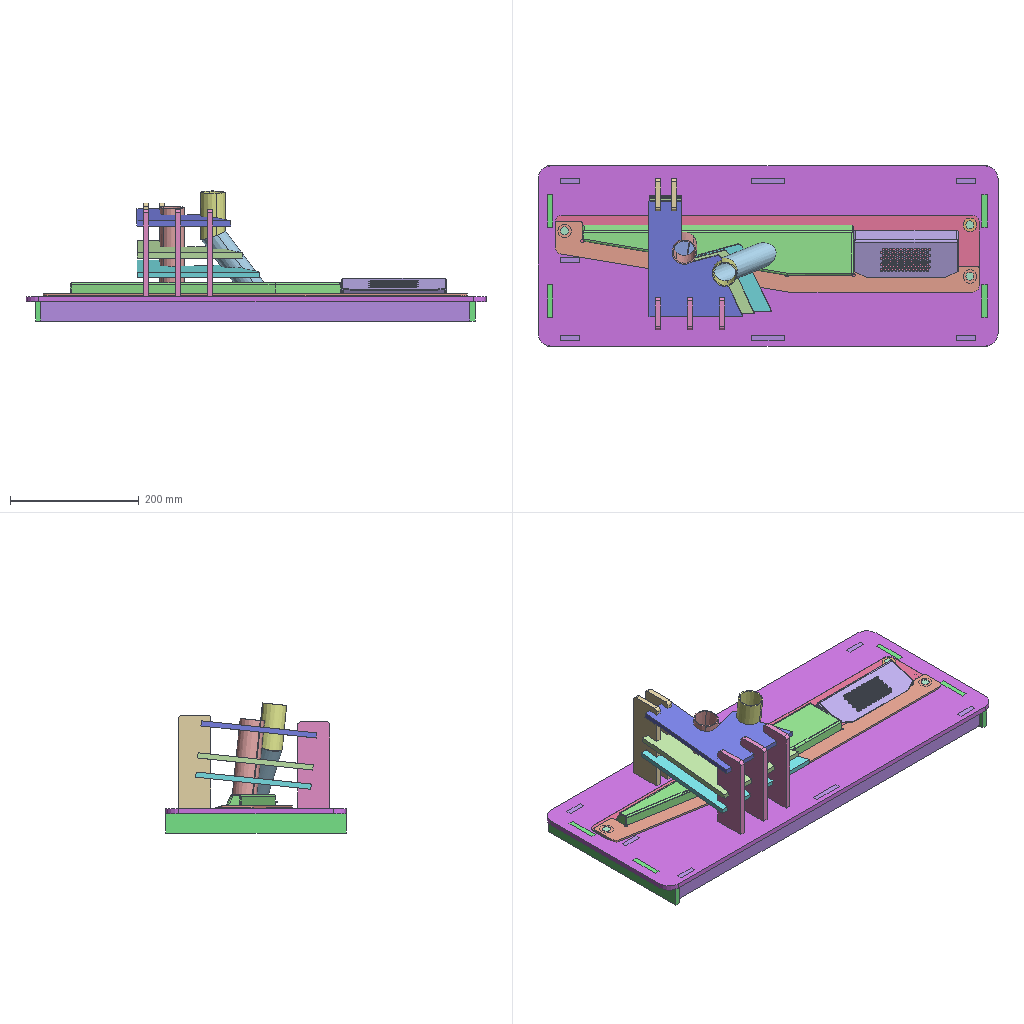Assembly | SolidWorks | 11 different items | 19 placed | box 715 x 280 x 202 mm
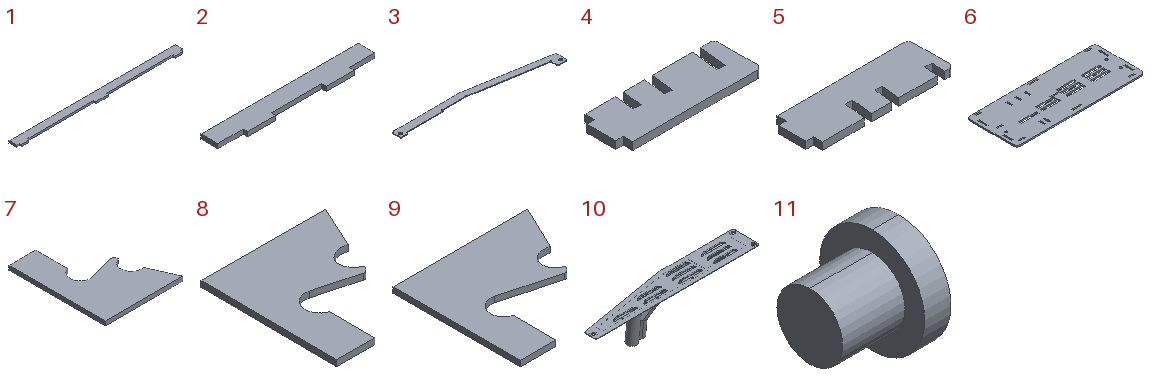Parts list (item | quantity | size | volume | features):
1 | x3 | 667 x 38 x 8 mm | 167120 mm3 | features FlatPattern 1, ICE 1, SMBaseFlange 1, SheetMetal 1
2 | x2 | 280 x 38 x 8 mm | 73600 mm3 | features FlatPattern 1, SMBaseFlange 1, SheetMetal 1
3 | x1 | 659 x 110.2 x 3 mm | 58163 mm3 | features Fillet 2, FlatPattern 1, SMBaseFlange 1, SheetMetal 1
4 | x3 | 143 x 50 x 8 mm | 51129 mm3 | features Fillet 1, FlatPattern 1, SMBaseFlange 1, SheetMetal 1
5 | x2 | 153 x 50 x 8 mm | 56042 mm3 | features Fillet 1, FlatPattern 1, SMBaseFlange 1, SheetMetal 1
6 | x1 | 715 x 280 x 8 mm | 1446309 mm3 | features FlatPattern 1, SMBaseFlange 1, SheetMetal 1
7 | x1 | 145.357 x 180 x 8 mm | 119080 mm3 | features FlatPattern 1, SMBaseFlange 1, SheetMetal 1
8 | x1 | 164.239 x 180.27 x 8 mm | 131142 mm3 | features FlatPattern 1, SMBaseFlange 1, SheetMetal 1
9 | x1 | 190.337 x 180 x 8 mm | 152502 mm3 | features FlatPattern 1, SMBaseFlange 1, SheetMetal 1
10 | x1 | 659 x 110.627 x 172.546 mm | 240293 mm3 | features BaseBody 11, ICE 1
11 | x3 | 16.9 x 20 x 20 mm | 3031 mm3 | features Revolution 1
Mates (type | each side: item.copy, entity, surface, feature):
InPlace | 10.1 face plane | 6.1 plane
InPlace | 11.1 plane | assembly plane
Concentric | 6.1 face cylinder Base-Flange1 | 11.2 face cylinder Revolve1
Coincident | 6.1 face plane Base-Flange1 | 11.2 face plane Revolve1
Concentric | 6.1 face cylinder Base-Flange1 | 11.3 face cylinder Revolve1
Coincident | 6.1 face plane Base-Flange1 | 11.3 face plane Revolve1
InPlace | 10.1 face plane | 3.1 plane
InPlace | 7.1 plane | assembly plane
InPlace | 8.1 plane | assembly plane
InPlace | 4.1 plane | assembly plane
DistanceDim | 9.1 face plane Base-Flange1 | 8.1 face plane Base-Flange1
Coincident | 8.1 face plane Base-Flange1 | 9.1 face plane Base-Flange1 | 2 times
InPlace | 5.1 plane | assembly plane
DistanceDim | 1.1 face plane Base-Flange1 | 6.1 face plane Base-Flange1
Coincident | 6.1 face plane Base-Flange1 | 1.1 face plane Base-Flange1
Coincident | 6.1 face plane Base-Flange1 | 2.1 face plane Base-Flange1 | 2 times
DistanceDim | 6.1 face plane Base-Flange1 | 2.1 face plane Base-Flange1